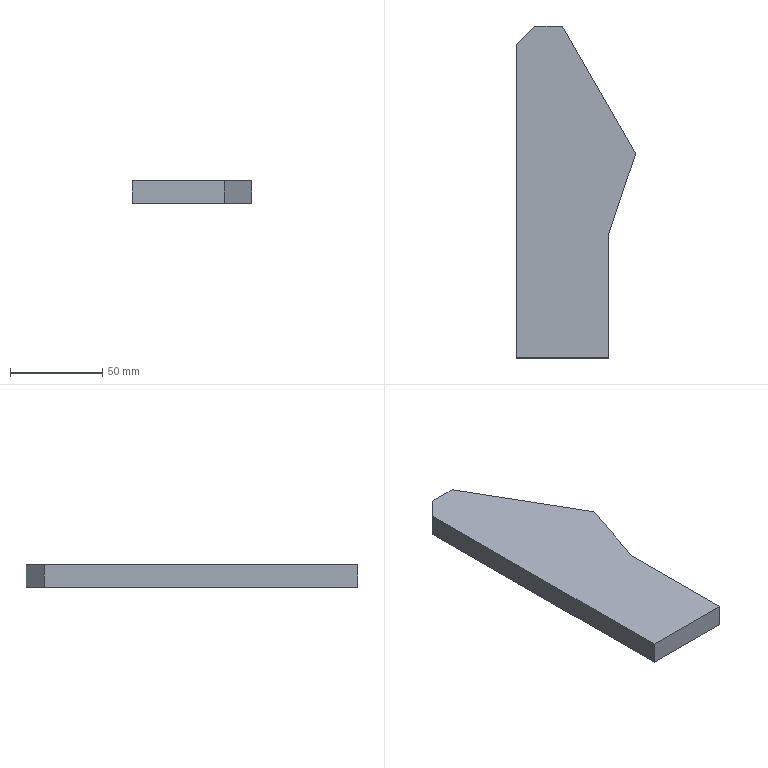Part | SolidWorks | features Chamfer 1, Extrusion 1 | 1 solid | 9 faces | box 64.77 x 180 x 12 mm | volume 107100 mm3 | plane 9
STEP:
#1=CARTESIAN_POINT('',(0.,0.,-6.));
#2=VERTEX_POINT('',#1);
#3=CARTESIAN_POINT('',(50.,0.,-6.));
#4=VERTEX_POINT('',#3);
#5=CARTESIAN_POINT('',(50.,0.,-6.));
#6=DIRECTION('',(1.,0.,0.));
#7=VECTOR('',#6,1000.);
#8=LINE('',#5,#7);
#9=EDGE_CURVE('',#2,#4,#8,.T.);
#10=ORIENTED_EDGE('',*,*,#9,.T.);
#11=CARTESIAN_POINT('',(50.,0.,6.));
#12=VERTEX_POINT('',#11);
#13=CARTESIAN_POINT('',(50.,0.,6.));
#14=DIRECTION('',(0.,0.,-1.));
#15=VECTOR('',#14,1000.);
#16=LINE('',#13,#15);
#17=EDGE_CURVE('',#12,#4,#16,.T.);
#18=ORIENTED_EDGE('',*,*,#17,.F.);
#19=CARTESIAN_POINT('',(0.,0.,6.));
#20=VERTEX_POINT('',#19);
#21=CARTESIAN_POINT('',(50.,0.,6.));
#22=DIRECTION('',(1.,0.,0.));
#23=VECTOR('',#22,1000.);
#24=LINE('',#21,#23);
#25=EDGE_CURVE('',#20,#12,#24,.T.);
#26=ORIENTED_EDGE('',*,*,#25,.F.);
#27=CARTESIAN_POINT('',(0.,0.,6.));
#28=DIRECTION('',(0.,0.,-1.));
#29=VECTOR('',#28,1000.);
#30=LINE('',#27,#29);
#31=EDGE_CURVE('',#20,#2,#30,.T.);
#32=ORIENTED_EDGE('',*,*,#31,.T.);
#33=EDGE_LOOP('',(#10,#18,#26,#32));
#34=FACE_OUTER_BOUND('',#33,.T.);
#35=CARTESIAN_POINT('',(50.,0.,6.));
#36=DIRECTION('',(0.,1.,0.));
#37=DIRECTION('',(-1.,0.,0.));
#38=AXIS2_PLACEMENT_3D('',#35,#36,#37);
#39=PLANE('',#38);
#40=ADVANCED_FACE('',(#34),#39,.F.);
#41=CARTESIAN_POINT('',(50.,66.792,-6.));
#42=VERTEX_POINT('',#41);
#43=CARTESIAN_POINT('',(50.,66.792,-6.));
#44=DIRECTION('',(0.,1.,0.));
#45=VECTOR('',#44,1000.);
#46=LINE('',#43,#45);
#47=EDGE_CURVE('',#4,#42,#46,.T.);
#48=ORIENTED_EDGE('',*,*,#47,.T.);
#49=CARTESIAN_POINT('',(50.,66.792,6.));
#50=VERTEX_POINT('',#49);
#51=CARTESIAN_POINT('',(50.,66.792,6.));
#52=DIRECTION('',(0.,0.,-1.));
#53=VECTOR('',#52,1000.);
#54=LINE('',#51,#53);
#55=EDGE_CURVE('',#50,#42,#54,.T.);
#56=ORIENTED_EDGE('',*,*,#55,.F.);
#57=CARTESIAN_POINT('',(50.,66.792,6.));
#58=DIRECTION('',(0.,1.,0.));
#59=VECTOR('',#58,1000.);
#60=LINE('',#57,#59);
#61=EDGE_CURVE('',#12,#50,#60,.T.);
#62=ORIENTED_EDGE('',*,*,#61,.F.);
#63=ORIENTED_EDGE('',*,*,#17,.T.);
#64=EDGE_LOOP('',(#48,#56,#62,#63));
#65=FACE_OUTER_BOUND('',#64,.T.);
#66=CARTESIAN_POINT('',(50.,66.792,6.));
#67=DIRECTION('',(-1.,0.,0.));
#68=DIRECTION('',(0.,-1.,0.));
#69=AXIS2_PLACEMENT_3D('',#66,#67,#68);
#70=PLANE('',#69);
#71=ADVANCED_FACE('',(#65),#70,.F.);
#72=CARTESIAN_POINT('',(64.77,111.116,-6.));
#73=VERTEX_POINT('',#72);
#74=CARTESIAN_POINT('',(64.77,111.116,-6.));
#75=DIRECTION('',(0.3161,0.9487,0.));
#76=VECTOR('',#75,1000.);
#77=LINE('',#74,#76);
#78=EDGE_CURVE('',#42,#73,#77,.T.);
#79=ORIENTED_EDGE('',*,*,#78,.T.);
#80=CARTESIAN_POINT('',(64.77,111.116,6.));
#81=VERTEX_POINT('',#80);
#82=CARTESIAN_POINT('',(64.77,111.116,6.));
#83=DIRECTION('',(0.,0.,-1.));
#84=VECTOR('',#83,1000.);
#85=LINE('',#82,#84);
#86=EDGE_CURVE('',#81,#73,#85,.T.);
#87=ORIENTED_EDGE('',*,*,#86,.F.);
#88=CARTESIAN_POINT('',(64.77,111.116,6.));
#89=DIRECTION('',(0.3161,0.9487,0.));
#90=VECTOR('',#89,1000.);
#91=LINE('',#88,#90);
#92=EDGE_CURVE('',#50,#81,#91,.T.);
#93=ORIENTED_EDGE('',*,*,#92,.F.);
#94=ORIENTED_EDGE('',*,*,#55,.T.);
#95=EDGE_LOOP('',(#79,#87,#93,#94));
#96=FACE_OUTER_BOUND('',#95,.T.);
#97=CARTESIAN_POINT('',(64.77,111.116,6.));
#98=DIRECTION('',(-0.9487,0.3161,0.));
#99=DIRECTION('',(-0.3161,-0.9487,0.));
#100=AXIS2_PLACEMENT_3D('',#97,#98,#99);
#101=PLANE('',#100);
#102=ADVANCED_FACE('',(#96),#101,.F.);
#103=CARTESIAN_POINT('',(25.,180.,-6.));
#104=VERTEX_POINT('',#103);
#105=CARTESIAN_POINT('',(25.,180.,-6.));
#106=DIRECTION('',(-0.5,0.866,0.));
#107=VECTOR('',#106,1000.);
#108=LINE('',#105,#107);
#109=EDGE_CURVE('',#73,#104,#108,.T.);
#110=ORIENTED_EDGE('',*,*,#109,.T.);
#111=CARTESIAN_POINT('',(25.,180.,6.));
#112=VERTEX_POINT('',#111);
#113=CARTESIAN_POINT('',(25.,180.,6.));
#114=DIRECTION('',(0.,0.,-1.));
#115=VECTOR('',#114,1000.);
#116=LINE('',#113,#115);
#117=EDGE_CURVE('',#112,#104,#116,.T.);
#118=ORIENTED_EDGE('',*,*,#117,.F.);
#119=CARTESIAN_POINT('',(25.,180.,6.));
#120=DIRECTION('',(-0.5,0.866,0.));
#121=VECTOR('',#120,1000.);
#122=LINE('',#119,#121);
#123=EDGE_CURVE('',#81,#112,#122,.T.);
#124=ORIENTED_EDGE('',*,*,#123,.F.);
#125=ORIENTED_EDGE('',*,*,#86,.T.);
#126=EDGE_LOOP('',(#110,#118,#124,#125));
#127=FACE_OUTER_BOUND('',#126,.T.);
#128=CARTESIAN_POINT('',(25.,180.,6.));
#129=DIRECTION('',(-0.866,-0.5,0.));
#130=DIRECTION('',(0.5,-0.866,0.));
#131=AXIS2_PLACEMENT_3D('',#128,#129,#130);
#132=PLANE('',#131);
#133=ADVANCED_FACE('',(#127),#132,.F.);
#134=CARTESIAN_POINT('',(10.,180.,-6.));
#135=VERTEX_POINT('',#134);
#136=CARTESIAN_POINT('',(0.,180.,-6.));
#137=DIRECTION('',(-1.,0.,0.));
#138=VECTOR('',#137,1000.);
#139=LINE('',#136,#138);
#140=EDGE_CURVE('',#104,#135,#139,.T.);
#141=ORIENTED_EDGE('',*,*,#140,.T.);
#142=CARTESIAN_POINT('',(10.,180.,6.));
#143=VERTEX_POINT('',#142);
#144=CARTESIAN_POINT('',(10.,180.,6.));
#145=DIRECTION('',(0.,0.,1.));
#146=VECTOR('',#145,1000.);
#147=LINE('',#144,#146);
#148=EDGE_CURVE('',#135,#143,#147,.T.);
#149=ORIENTED_EDGE('',*,*,#148,.T.);
#150=CARTESIAN_POINT('',(0.,180.,6.));
#151=DIRECTION('',(-1.,0.,0.));
#152=VECTOR('',#151,1000.);
#153=LINE('',#150,#152);
#154=EDGE_CURVE('',#112,#143,#153,.T.);
#155=ORIENTED_EDGE('',*,*,#154,.F.);
#156=ORIENTED_EDGE('',*,*,#117,.T.);
#157=EDGE_LOOP('',(#141,#149,#155,#156));
#158=FACE_OUTER_BOUND('',#157,.T.);
#159=CARTESIAN_POINT('',(0.,180.,6.));
#160=DIRECTION('',(0.,-1.,0.));
#161=DIRECTION('',(0.,0.,-1.));
#162=AXIS2_PLACEMENT_3D('',#159,#160,#161);
#163=PLANE('',#162);
#164=ADVANCED_FACE('',(#158),#163,.F.);
#165=CARTESIAN_POINT('',(0.,170.,6.));
#166=VERTEX_POINT('',#165);
#167=CARTESIAN_POINT('',(0.,0.,6.));
#168=DIRECTION('',(0.,-1.,0.));
#169=VECTOR('',#168,1000.);
#170=LINE('',#167,#169);
#171=EDGE_CURVE('',#166,#20,#170,.T.);
#172=ORIENTED_EDGE('',*,*,#171,.F.);
#173=CARTESIAN_POINT('',(0.,170.,-6.));
#174=VERTEX_POINT('',#173);
#175=CARTESIAN_POINT('',(0.,170.,6.));
#176=DIRECTION('',(0.,0.,-1.));
#177=VECTOR('',#176,1000.);
#178=LINE('',#175,#177);
#179=EDGE_CURVE('',#166,#174,#178,.T.);
#180=ORIENTED_EDGE('',*,*,#179,.T.);
#181=CARTESIAN_POINT('',(0.,0.,-6.));
#182=DIRECTION('',(0.,-1.,0.));
#183=VECTOR('',#182,1000.);
#184=LINE('',#181,#183);
#185=EDGE_CURVE('',#174,#2,#184,.T.);
#186=ORIENTED_EDGE('',*,*,#185,.T.);
#187=ORIENTED_EDGE('',*,*,#31,.F.);
#188=EDGE_LOOP('',(#172,#180,#186,#187));
#189=FACE_OUTER_BOUND('',#188,.T.);
#190=CARTESIAN_POINT('',(0.,0.,6.));
#191=DIRECTION('',(1.,0.,0.));
#192=DIRECTION('',(0.,0.,-1.));
#193=AXIS2_PLACEMENT_3D('',#190,#191,#192);
#194=PLANE('',#193);
#195=ADVANCED_FACE('',(#189),#194,.F.);
#196=ORIENTED_EDGE('',*,*,#154,.T.);
#197=CARTESIAN_POINT('',(0.,170.,6.));
#198=DIRECTION('',(-0.7071,-0.7071,0.));
#199=VECTOR('',#198,1000.);
#200=LINE('',#197,#199);
#201=EDGE_CURVE('',#143,#166,#200,.T.);
#202=ORIENTED_EDGE('',*,*,#201,.T.);
#203=ORIENTED_EDGE('',*,*,#171,.T.);
#204=ORIENTED_EDGE('',*,*,#25,.T.);
#205=ORIENTED_EDGE('',*,*,#61,.T.);
#206=ORIENTED_EDGE('',*,*,#92,.T.);
#207=ORIENTED_EDGE('',*,*,#123,.T.);
#208=EDGE_LOOP('',(#196,#202,#203,#204,#205,#206,#207));
#209=FACE_OUTER_BOUND('',#208,.T.);
#210=CARTESIAN_POINT('',(0.,0.,6.));
#211=DIRECTION('',(0.,0.,-1.));
#212=DIRECTION('',(-1.,0.,0.));
#213=AXIS2_PLACEMENT_3D('',#210,#211,#212);
#214=PLANE('',#213);
#215=ADVANCED_FACE('',(#209),#214,.F.);
#216=ORIENTED_EDGE('',*,*,#185,.F.);
#217=CARTESIAN_POINT('',(-85.,85.,-6.));
#218=DIRECTION('',(0.7071,0.7071,0.));
#219=VECTOR('',#218,1000.);
#220=LINE('',#217,#219);
#221=EDGE_CURVE('',#174,#135,#220,.T.);
#222=ORIENTED_EDGE('',*,*,#221,.T.);
#223=ORIENTED_EDGE('',*,*,#140,.F.);
#224=ORIENTED_EDGE('',*,*,#109,.F.);
#225=ORIENTED_EDGE('',*,*,#78,.F.);
#226=ORIENTED_EDGE('',*,*,#47,.F.);
#227=ORIENTED_EDGE('',*,*,#9,.F.);
#228=EDGE_LOOP('',(#216,#222,#223,#224,#225,#226,#227));
#229=FACE_OUTER_BOUND('',#228,.T.);
#230=CARTESIAN_POINT('',(0.,0.,-6.));
#231=DIRECTION('',(0.,0.,-1.));
#232=DIRECTION('',(-1.,0.,0.));
#233=AXIS2_PLACEMENT_3D('',#230,#231,#232);
#234=PLANE('',#233);
#235=ADVANCED_FACE('',(#229),#234,.T.);
#236=ORIENTED_EDGE('',*,*,#201,.F.);
#237=ORIENTED_EDGE('',*,*,#148,.F.);
#238=ORIENTED_EDGE('',*,*,#221,.F.);
#239=ORIENTED_EDGE('',*,*,#179,.F.);
#240=EDGE_LOOP('',(#236,#237,#238,#239));
#241=FACE_OUTER_BOUND('',#240,.T.);
#242=CARTESIAN_POINT('',(0.,170.,6.));
#243=DIRECTION('',(0.7071,-0.7071,0.));
#244=DIRECTION('',(0.,0.,-1.));
#245=AXIS2_PLACEMENT_3D('',#242,#243,#244);
#246=PLANE('',#245);
#247=ADVANCED_FACE('',(#241),#246,.F.);
#248=CLOSED_SHELL('',(#40,#71,#102,#133,#164,#195,#215,#235,#247));
#249=MANIFOLD_SOLID_BREP('',#248);
#250=CARTESIAN_POINT('',(0.,0.,0.));
#251=DIRECTION('',(0.,0.,1.));
#252=DIRECTION('',(1.,0.,0.));
#253=AXIS2_PLACEMENT_3D('',#250,#251,#252);
#254=(LENGTH_UNIT()NAMED_UNIT(*)SI_UNIT(.MILLI.,.METRE.));
#255=UNCERTAINTY_MEASURE_WITH_UNIT(LENGTH_MEASURE(0.00001),#254,'','');
#256=(NAMED_UNIT(*)PLANE_ANGLE_UNIT()SI_UNIT($,.RADIAN.));
#257=(NAMED_UNIT(*)SI_UNIT($,.STERADIAN.)SOLID_ANGLE_UNIT());
#258=(GEOMETRIC_REPRESENTATION_CONTEXT(3)GLOBAL_UNCERTAINTY_ASSIGNED_CONTEXT((#255))GLOBAL_UNIT_ASSIGNED_CONTEXT((#254,#256,#257))REPRESENTATION_CONTEXT('',''));
#259=ADVANCED_BREP_SHAPE_REPRESENTATION('',(#249,#253),#258);